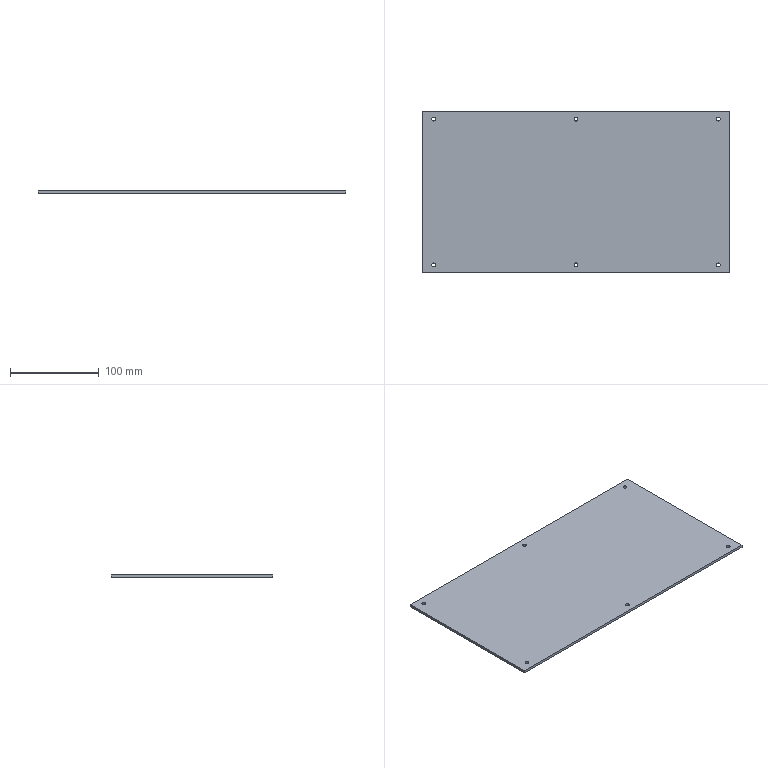Part | SolidWorks | features Cut 1, Extrusion 1 | 1 solid | 18 faces | box 346 x 182 x 3 mm | volume 188642 mm3 | cylinder 12 | plane 6 | commonest cylinder face diameters 4.4 x12
STEP:
#1=CARTESIAN_POINT('',(157.8,-82.,3.));
#2=VERTEX_POINT('',#1);
#3=CARTESIAN_POINT('',(162.2,-82.,3.));
#4=VERTEX_POINT('',#3);
#5=CARTESIAN_POINT('',(160.,-82.,3.));
#6=DIRECTION('',(0.,0.,1.));
#7=DIRECTION('',(1.,0.,0.));
#8=AXIS2_PLACEMENT_3D('',#5,#6,#7);
#9=CIRCLE('',#8,2.2);
#10=EDGE_CURVE('',#2,#4,#9,.T.);
#11=ORIENTED_EDGE('',*,*,#10,.T.);
#12=CARTESIAN_POINT('',(162.2,-82.,0.));
#13=VERTEX_POINT('',#12);
#14=CARTESIAN_POINT('',(162.2,-82.,10.));
#15=DIRECTION('',(0.,0.,-1.));
#16=VECTOR('',#15,1000.);
#17=LINE('',#14,#16);
#18=EDGE_CURVE('',#4,#13,#17,.T.);
#19=ORIENTED_EDGE('',*,*,#18,.T.);
#20=CARTESIAN_POINT('',(157.8,-82.,0.));
#21=VERTEX_POINT('',#20);
#22=CARTESIAN_POINT('',(160.,-82.,0.));
#23=DIRECTION('',(0.,0.,-1.));
#24=DIRECTION('',(-1.,0.,0.));
#25=AXIS2_PLACEMENT_3D('',#22,#23,#24);
#26=CIRCLE('',#25,2.2);
#27=EDGE_CURVE('',#13,#21,#26,.T.);
#28=ORIENTED_EDGE('',*,*,#27,.T.);
#29=CARTESIAN_POINT('',(157.8,-82.,10.));
#30=DIRECTION('',(0.,0.,-1.));
#31=VECTOR('',#30,1000.);
#32=LINE('',#29,#31);
#33=EDGE_CURVE('',#2,#21,#32,.T.);
#34=ORIENTED_EDGE('',*,*,#33,.F.);
#35=EDGE_LOOP('',(#11,#19,#28,#34));
#36=FACE_OUTER_BOUND('',#35,.T.);
#37=CARTESIAN_POINT('',(160.,-82.,10.));
#38=DIRECTION('',(0.,0.,-1.));
#39=DIRECTION('',(-1.,0.,0.));
#40=AXIS2_PLACEMENT_3D('',#37,#38,#39);
#41=CYLINDRICAL_SURFACE('',#40,2.2);
#42=ADVANCED_FACE('',(#36),#41,.F.);
#43=CARTESIAN_POINT('',(-162.2,-82.,3.));
#44=VERTEX_POINT('',#43);
#45=CARTESIAN_POINT('',(-157.8,-82.,3.));
#46=VERTEX_POINT('',#45);
#47=CARTESIAN_POINT('',(-160.,-82.,3.));
#48=DIRECTION('',(0.,0.,1.));
#49=DIRECTION('',(1.,0.,0.));
#50=AXIS2_PLACEMENT_3D('',#47,#48,#49);
#51=CIRCLE('',#50,2.2);
#52=EDGE_CURVE('',#44,#46,#51,.T.);
#53=ORIENTED_EDGE('',*,*,#52,.T.);
#54=CARTESIAN_POINT('',(-157.8,-82.,0.));
#55=VERTEX_POINT('',#54);
#56=CARTESIAN_POINT('',(-157.8,-82.,10.));
#57=DIRECTION('',(0.,0.,-1.));
#58=VECTOR('',#57,1000.);
#59=LINE('',#56,#58);
#60=EDGE_CURVE('',#46,#55,#59,.T.);
#61=ORIENTED_EDGE('',*,*,#60,.T.);
#62=CARTESIAN_POINT('',(-162.2,-82.,0.));
#63=VERTEX_POINT('',#62);
#64=CARTESIAN_POINT('',(-160.,-82.,0.));
#65=DIRECTION('',(0.,0.,-1.));
#66=DIRECTION('',(-1.,0.,0.));
#67=AXIS2_PLACEMENT_3D('',#64,#65,#66);
#68=CIRCLE('',#67,2.2);
#69=EDGE_CURVE('',#55,#63,#68,.T.);
#70=ORIENTED_EDGE('',*,*,#69,.T.);
#71=CARTESIAN_POINT('',(-162.2,-82.,10.));
#72=DIRECTION('',(0.,0.,-1.));
#73=VECTOR('',#72,1000.);
#74=LINE('',#71,#73);
#75=EDGE_CURVE('',#44,#63,#74,.T.);
#76=ORIENTED_EDGE('',*,*,#75,.F.);
#77=EDGE_LOOP('',(#53,#61,#70,#76));
#78=FACE_OUTER_BOUND('',#77,.T.);
#79=CARTESIAN_POINT('',(-160.,-82.,10.));
#80=DIRECTION('',(0.,0.,-1.));
#81=DIRECTION('',(-1.,0.,0.));
#82=AXIS2_PLACEMENT_3D('',#79,#80,#81);
#83=CYLINDRICAL_SURFACE('',#82,2.2);
#84=ADVANCED_FACE('',(#78),#83,.F.);
#85=CARTESIAN_POINT('',(-2.2,-82.,3.));
#86=VERTEX_POINT('',#85);
#87=CARTESIAN_POINT('',(2.2,-82.,3.));
#88=VERTEX_POINT('',#87);
#89=CARTESIAN_POINT('',(0.,-82.,3.));
#90=DIRECTION('',(0.,0.,1.));
#91=DIRECTION('',(1.,0.,0.));
#92=AXIS2_PLACEMENT_3D('',#89,#90,#91);
#93=CIRCLE('',#92,2.2);
#94=EDGE_CURVE('',#86,#88,#93,.T.);
#95=ORIENTED_EDGE('',*,*,#94,.T.);
#96=CARTESIAN_POINT('',(2.2,-82.,0.));
#97=VERTEX_POINT('',#96);
#98=CARTESIAN_POINT('',(2.2,-82.,10.));
#99=DIRECTION('',(0.,0.,-1.));
#100=VECTOR('',#99,1000.);
#101=LINE('',#98,#100);
#102=EDGE_CURVE('',#88,#97,#101,.T.);
#103=ORIENTED_EDGE('',*,*,#102,.T.);
#104=CARTESIAN_POINT('',(-2.2,-82.,0.));
#105=VERTEX_POINT('',#104);
#106=CARTESIAN_POINT('',(0.,-82.,0.));
#107=DIRECTION('',(0.,0.,-1.));
#108=DIRECTION('',(-1.,0.,0.));
#109=AXIS2_PLACEMENT_3D('',#106,#107,#108);
#110=CIRCLE('',#109,2.2);
#111=EDGE_CURVE('',#97,#105,#110,.T.);
#112=ORIENTED_EDGE('',*,*,#111,.T.);
#113=CARTESIAN_POINT('',(-2.2,-82.,10.));
#114=DIRECTION('',(0.,0.,-1.));
#115=VECTOR('',#114,1000.);
#116=LINE('',#113,#115);
#117=EDGE_CURVE('',#86,#105,#116,.T.);
#118=ORIENTED_EDGE('',*,*,#117,.F.);
#119=EDGE_LOOP('',(#95,#103,#112,#118));
#120=FACE_OUTER_BOUND('',#119,.T.);
#121=CARTESIAN_POINT('',(0.,-82.,10.));
#122=DIRECTION('',(0.,0.,-1.));
#123=DIRECTION('',(-1.,0.,0.));
#124=AXIS2_PLACEMENT_3D('',#121,#122,#123);
#125=CYLINDRICAL_SURFACE('',#124,2.2);
#126=ADVANCED_FACE('',(#120),#125,.F.);
#127=CARTESIAN_POINT('',(-162.2,82.,3.));
#128=VERTEX_POINT('',#127);
#129=CARTESIAN_POINT('',(-157.8,82.,3.));
#130=VERTEX_POINT('',#129);
#131=CARTESIAN_POINT('',(-160.,82.,3.));
#132=DIRECTION('',(0.,0.,1.));
#133=DIRECTION('',(1.,0.,0.));
#134=AXIS2_PLACEMENT_3D('',#131,#132,#133);
#135=CIRCLE('',#134,2.2);
#136=EDGE_CURVE('',#128,#130,#135,.T.);
#137=ORIENTED_EDGE('',*,*,#136,.T.);
#138=CARTESIAN_POINT('',(-157.8,82.,0.));
#139=VERTEX_POINT('',#138);
#140=CARTESIAN_POINT('',(-157.8,82.,10.));
#141=DIRECTION('',(0.,0.,-1.));
#142=VECTOR('',#141,1000.);
#143=LINE('',#140,#142);
#144=EDGE_CURVE('',#130,#139,#143,.T.);
#145=ORIENTED_EDGE('',*,*,#144,.T.);
#146=CARTESIAN_POINT('',(-162.2,82.,0.));
#147=VERTEX_POINT('',#146);
#148=CARTESIAN_POINT('',(-160.,82.,0.));
#149=DIRECTION('',(0.,0.,-1.));
#150=DIRECTION('',(-1.,0.,0.));
#151=AXIS2_PLACEMENT_3D('',#148,#149,#150);
#152=CIRCLE('',#151,2.2);
#153=EDGE_CURVE('',#139,#147,#152,.T.);
#154=ORIENTED_EDGE('',*,*,#153,.T.);
#155=CARTESIAN_POINT('',(-162.2,82.,10.));
#156=DIRECTION('',(0.,0.,-1.));
#157=VECTOR('',#156,1000.);
#158=LINE('',#155,#157);
#159=EDGE_CURVE('',#128,#147,#158,.T.);
#160=ORIENTED_EDGE('',*,*,#159,.F.);
#161=EDGE_LOOP('',(#137,#145,#154,#160));
#162=FACE_OUTER_BOUND('',#161,.T.);
#163=CARTESIAN_POINT('',(-160.,82.,10.));
#164=DIRECTION('',(0.,0.,-1.));
#165=DIRECTION('',(-1.,0.,0.));
#166=AXIS2_PLACEMENT_3D('',#163,#164,#165);
#167=CYLINDRICAL_SURFACE('',#166,2.2);
#168=ADVANCED_FACE('',(#162),#167,.F.);
#169=CARTESIAN_POINT('',(-2.2,82.,3.));
#170=VERTEX_POINT('',#169);
#171=CARTESIAN_POINT('',(2.2,82.,3.));
#172=VERTEX_POINT('',#171);
#173=CARTESIAN_POINT('',(0.,82.,3.));
#174=DIRECTION('',(0.,0.,1.));
#175=DIRECTION('',(1.,0.,0.));
#176=AXIS2_PLACEMENT_3D('',#173,#174,#175);
#177=CIRCLE('',#176,2.2);
#178=EDGE_CURVE('',#170,#172,#177,.T.);
#179=ORIENTED_EDGE('',*,*,#178,.T.);
#180=CARTESIAN_POINT('',(2.2,82.,0.));
#181=VERTEX_POINT('',#180);
#182=CARTESIAN_POINT('',(2.2,82.,10.));
#183=DIRECTION('',(0.,0.,-1.));
#184=VECTOR('',#183,1000.);
#185=LINE('',#182,#184);
#186=EDGE_CURVE('',#172,#181,#185,.T.);
#187=ORIENTED_EDGE('',*,*,#186,.T.);
#188=CARTESIAN_POINT('',(-2.2,82.,0.));
#189=VERTEX_POINT('',#188);
#190=CARTESIAN_POINT('',(0.,82.,0.));
#191=DIRECTION('',(0.,0.,-1.));
#192=DIRECTION('',(-1.,0.,0.));
#193=AXIS2_PLACEMENT_3D('',#190,#191,#192);
#194=CIRCLE('',#193,2.2);
#195=EDGE_CURVE('',#181,#189,#194,.T.);
#196=ORIENTED_EDGE('',*,*,#195,.T.);
#197=CARTESIAN_POINT('',(-2.2,82.,10.));
#198=DIRECTION('',(0.,0.,-1.));
#199=VECTOR('',#198,1000.);
#200=LINE('',#197,#199);
#201=EDGE_CURVE('',#170,#189,#200,.T.);
#202=ORIENTED_EDGE('',*,*,#201,.F.);
#203=EDGE_LOOP('',(#179,#187,#196,#202));
#204=FACE_OUTER_BOUND('',#203,.T.);
#205=CARTESIAN_POINT('',(0.,82.,10.));
#206=DIRECTION('',(0.,0.,-1.));
#207=DIRECTION('',(-1.,0.,0.));
#208=AXIS2_PLACEMENT_3D('',#205,#206,#207);
#209=CYLINDRICAL_SURFACE('',#208,2.2);
#210=ADVANCED_FACE('',(#204),#209,.F.);
#211=CARTESIAN_POINT('',(157.8,82.,3.));
#212=VERTEX_POINT('',#211);
#213=CARTESIAN_POINT('',(162.2,82.,3.));
#214=VERTEX_POINT('',#213);
#215=CARTESIAN_POINT('',(160.,82.,3.));
#216=DIRECTION('',(0.,0.,1.));
#217=DIRECTION('',(1.,0.,0.));
#218=AXIS2_PLACEMENT_3D('',#215,#216,#217);
#219=CIRCLE('',#218,2.2);
#220=EDGE_CURVE('',#212,#214,#219,.T.);
#221=ORIENTED_EDGE('',*,*,#220,.T.);
#222=CARTESIAN_POINT('',(162.2,82.,0.));
#223=VERTEX_POINT('',#222);
#224=CARTESIAN_POINT('',(162.2,82.,10.));
#225=DIRECTION('',(0.,0.,-1.));
#226=VECTOR('',#225,1000.);
#227=LINE('',#224,#226);
#228=EDGE_CURVE('',#214,#223,#227,.T.);
#229=ORIENTED_EDGE('',*,*,#228,.T.);
#230=CARTESIAN_POINT('',(157.8,82.,0.));
#231=VERTEX_POINT('',#230);
#232=CARTESIAN_POINT('',(160.,82.,0.));
#233=DIRECTION('',(0.,0.,-1.));
#234=DIRECTION('',(-1.,0.,0.));
#235=AXIS2_PLACEMENT_3D('',#232,#233,#234);
#236=CIRCLE('',#235,2.2);
#237=EDGE_CURVE('',#223,#231,#236,.T.);
#238=ORIENTED_EDGE('',*,*,#237,.T.);
#239=CARTESIAN_POINT('',(157.8,82.,10.));
#240=DIRECTION('',(0.,0.,-1.));
#241=VECTOR('',#240,1000.);
#242=LINE('',#239,#241);
#243=EDGE_CURVE('',#212,#231,#242,.T.);
#244=ORIENTED_EDGE('',*,*,#243,.F.);
#245=EDGE_LOOP('',(#221,#229,#238,#244));
#246=FACE_OUTER_BOUND('',#245,.T.);
#247=CARTESIAN_POINT('',(160.,82.,10.));
#248=DIRECTION('',(0.,0.,-1.));
#249=DIRECTION('',(-1.,0.,0.));
#250=AXIS2_PLACEMENT_3D('',#247,#248,#249);
#251=CYLINDRICAL_SURFACE('',#250,2.2);
#252=ADVANCED_FACE('',(#246),#251,.F.);
#253=CARTESIAN_POINT('',(-173.,91.,0.));
#254=VERTEX_POINT('',#253);
#255=CARTESIAN_POINT('',(-173.,-91.,0.));
#256=VERTEX_POINT('',#255);
#257=CARTESIAN_POINT('',(-173.,-91.,0.));
#258=DIRECTION('',(0.,-1.,0.));
#259=VECTOR('',#258,1000.);
#260=LINE('',#257,#259);
#261=EDGE_CURVE('',#254,#256,#260,.T.);
#262=ORIENTED_EDGE('',*,*,#261,.T.);
#263=CARTESIAN_POINT('',(-173.,-91.,3.));
#264=VERTEX_POINT('',#263);
#265=CARTESIAN_POINT('',(-173.,-91.,3.));
#266=DIRECTION('',(0.,0.,-1.));
#267=VECTOR('',#266,1000.);
#268=LINE('',#265,#267);
#269=EDGE_CURVE('',#264,#256,#268,.T.);
#270=ORIENTED_EDGE('',*,*,#269,.F.);
#271=CARTESIAN_POINT('',(-173.,91.,3.));
#272=VERTEX_POINT('',#271);
#273=CARTESIAN_POINT('',(-173.,-91.,3.));
#274=DIRECTION('',(0.,-1.,0.));
#275=VECTOR('',#274,1000.);
#276=LINE('',#273,#275);
#277=EDGE_CURVE('',#272,#264,#276,.T.);
#278=ORIENTED_EDGE('',*,*,#277,.F.);
#279=CARTESIAN_POINT('',(-173.,91.,3.));
#280=DIRECTION('',(0.,0.,-1.));
#281=VECTOR('',#280,1000.);
#282=LINE('',#279,#281);
#283=EDGE_CURVE('',#272,#254,#282,.T.);
#284=ORIENTED_EDGE('',*,*,#283,.T.);
#285=EDGE_LOOP('',(#262,#270,#278,#284));
#286=FACE_OUTER_BOUND('',#285,.T.);
#287=CARTESIAN_POINT('',(-173.,-91.,3.));
#288=DIRECTION('',(1.,0.,0.));
#289=DIRECTION('',(0.,0.,-1.));
#290=AXIS2_PLACEMENT_3D('',#287,#288,#289);
#291=PLANE('',#290);
#292=ADVANCED_FACE('',(#286),#291,.F.);
#293=CARTESIAN_POINT('',(173.,-91.,0.));
#294=VERTEX_POINT('',#293);
#295=CARTESIAN_POINT('',(173.,-91.,0.));
#296=DIRECTION('',(1.,0.,0.));
#297=VECTOR('',#296,1000.);
#298=LINE('',#295,#297);
#299=EDGE_CURVE('',#256,#294,#298,.T.);
#300=ORIENTED_EDGE('',*,*,#299,.T.);
#301=CARTESIAN_POINT('',(173.,-91.,3.));
#302=VERTEX_POINT('',#301);
#303=CARTESIAN_POINT('',(173.,-91.,3.));
#304=DIRECTION('',(0.,0.,-1.));
#305=VECTOR('',#304,1000.);
#306=LINE('',#303,#305);
#307=EDGE_CURVE('',#302,#294,#306,.T.);
#308=ORIENTED_EDGE('',*,*,#307,.F.);
#309=CARTESIAN_POINT('',(173.,-91.,3.));
#310=DIRECTION('',(1.,0.,0.));
#311=VECTOR('',#310,1000.);
#312=LINE('',#309,#311);
#313=EDGE_CURVE('',#264,#302,#312,.T.);
#314=ORIENTED_EDGE('',*,*,#313,.F.);
#315=ORIENTED_EDGE('',*,*,#269,.T.);
#316=EDGE_LOOP('',(#300,#308,#314,#315));
#317=FACE_OUTER_BOUND('',#316,.T.);
#318=CARTESIAN_POINT('',(173.,-91.,3.));
#319=DIRECTION('',(0.,1.,0.));
#320=DIRECTION('',(-1.,0.,0.));
#321=AXIS2_PLACEMENT_3D('',#318,#319,#320);
#322=PLANE('',#321);
#323=ADVANCED_FACE('',(#317),#322,.F.);
#324=CARTESIAN_POINT('',(173.,91.,0.));
#325=VERTEX_POINT('',#324);
#326=CARTESIAN_POINT('',(173.,-91.,0.));
#327=DIRECTION('',(0.,1.,0.));
#328=VECTOR('',#327,1000.);
#329=LINE('',#326,#328);
#330=EDGE_CURVE('',#294,#325,#329,.T.);
#331=ORIENTED_EDGE('',*,*,#330,.T.);
#332=CARTESIAN_POINT('',(173.,91.,3.));
#333=VERTEX_POINT('',#332);
#334=CARTESIAN_POINT('',(173.,91.,3.));
#335=DIRECTION('',(0.,0.,-1.));
#336=VECTOR('',#335,1000.);
#337=LINE('',#334,#336);
#338=EDGE_CURVE('',#333,#325,#337,.T.);
#339=ORIENTED_EDGE('',*,*,#338,.F.);
#340=CARTESIAN_POINT('',(173.,-91.,3.));
#341=DIRECTION('',(0.,1.,0.));
#342=VECTOR('',#341,1000.);
#343=LINE('',#340,#342);
#344=EDGE_CURVE('',#302,#333,#343,.T.);
#345=ORIENTED_EDGE('',*,*,#344,.F.);
#346=ORIENTED_EDGE('',*,*,#307,.T.);
#347=EDGE_LOOP('',(#331,#339,#345,#346));
#348=FACE_OUTER_BOUND('',#347,.T.);
#349=CARTESIAN_POINT('',(173.,-91.,3.));
#350=DIRECTION('',(-1.,0.,0.));
#351=DIRECTION('',(0.,0.,1.));
#352=AXIS2_PLACEMENT_3D('',#349,#350,#351);
#353=PLANE('',#352);
#354=ADVANCED_FACE('',(#348),#353,.F.);
#355=CARTESIAN_POINT('',(173.,91.,0.));
#356=DIRECTION('',(-1.,0.,0.));
#357=VECTOR('',#356,1000.);
#358=LINE('',#355,#357);
#359=EDGE_CURVE('',#325,#254,#358,.T.);
#360=ORIENTED_EDGE('',*,*,#359,.T.);
#361=ORIENTED_EDGE('',*,*,#283,.F.);
#362=CARTESIAN_POINT('',(173.,91.,3.));
#363=DIRECTION('',(-1.,0.,0.));
#364=VECTOR('',#363,1000.);
#365=LINE('',#362,#364);
#366=EDGE_CURVE('',#333,#272,#365,.T.);
#367=ORIENTED_EDGE('',*,*,#366,.F.);
#368=ORIENTED_EDGE('',*,*,#338,.T.);
#369=EDGE_LOOP('',(#360,#361,#367,#368));
#370=FACE_OUTER_BOUND('',#369,.T.);
#371=CARTESIAN_POINT('',(173.,91.,3.));
#372=DIRECTION('',(0.,-1.,0.));
#373=DIRECTION('',(1.,0.,0.));
#374=AXIS2_PLACEMENT_3D('',#371,#372,#373);
#375=PLANE('',#374);
#376=ADVANCED_FACE('',(#370),#375,.F.);
#377=ORIENTED_EDGE('',*,*,#10,.F.);
#378=CARTESIAN_POINT('',(160.,-82.,3.));
#379=DIRECTION('',(0.,0.,1.));
#380=DIRECTION('',(1.,0.,0.));
#381=AXIS2_PLACEMENT_3D('',#378,#379,#380);
#382=CIRCLE('',#381,2.2);
#383=EDGE_CURVE('',#4,#2,#382,.T.);
#384=ORIENTED_EDGE('',*,*,#383,.F.);
#385=EDGE_LOOP('',(#377,#384));
#386=FACE_BOUND('',#385,.T.);
#387=ORIENTED_EDGE('',*,*,#52,.F.);
#388=CARTESIAN_POINT('',(-160.,-82.,3.));
#389=DIRECTION('',(0.,0.,1.));
#390=DIRECTION('',(1.,0.,0.));
#391=AXIS2_PLACEMENT_3D('',#388,#389,#390);
#392=CIRCLE('',#391,2.2);
#393=EDGE_CURVE('',#46,#44,#392,.T.);
#394=ORIENTED_EDGE('',*,*,#393,.F.);
#395=EDGE_LOOP('',(#387,#394));
#396=FACE_BOUND('',#395,.T.);
#397=ORIENTED_EDGE('',*,*,#94,.F.);
#398=CARTESIAN_POINT('',(0.,-82.,3.));
#399=DIRECTION('',(0.,0.,1.));
#400=DIRECTION('',(1.,0.,0.));
#401=AXIS2_PLACEMENT_3D('',#398,#399,#400);
#402=CIRCLE('',#401,2.2);
#403=EDGE_CURVE('',#88,#86,#402,.T.);
#404=ORIENTED_EDGE('',*,*,#403,.F.);
#405=EDGE_LOOP('',(#397,#404));
#406=FACE_BOUND('',#405,.T.);
#407=ORIENTED_EDGE('',*,*,#136,.F.);
#408=CARTESIAN_POINT('',(-160.,82.,3.));
#409=DIRECTION('',(0.,0.,1.));
#410=DIRECTION('',(1.,0.,0.));
#411=AXIS2_PLACEMENT_3D('',#408,#409,#410);
#412=CIRCLE('',#411,2.2);
#413=EDGE_CURVE('',#130,#128,#412,.T.);
#414=ORIENTED_EDGE('',*,*,#413,.F.);
#415=EDGE_LOOP('',(#407,#414));
#416=FACE_BOUND('',#415,.T.);
#417=ORIENTED_EDGE('',*,*,#178,.F.);
#418=CARTESIAN_POINT('',(0.,82.,3.));
#419=DIRECTION('',(0.,0.,1.));
#420=DIRECTION('',(1.,0.,0.));
#421=AXIS2_PLACEMENT_3D('',#418,#419,#420);
#422=CIRCLE('',#421,2.2);
#423=EDGE_CURVE('',#172,#170,#422,.T.);
#424=ORIENTED_EDGE('',*,*,#423,.F.);
#425=EDGE_LOOP('',(#417,#424));
#426=FACE_BOUND('',#425,.T.);
#427=ORIENTED_EDGE('',*,*,#220,.F.);
#428=CARTESIAN_POINT('',(160.,82.,3.));
#429=DIRECTION('',(0.,0.,1.));
#430=DIRECTION('',(1.,0.,0.));
#431=AXIS2_PLACEMENT_3D('',#428,#429,#430);
#432=CIRCLE('',#431,2.2);
#433=EDGE_CURVE('',#214,#212,#432,.T.);
#434=ORIENTED_EDGE('',*,*,#433,.F.);
#435=EDGE_LOOP('',(#427,#434));
#436=FACE_BOUND('',#435,.T.);
#437=ORIENTED_EDGE('',*,*,#277,.T.);
#438=ORIENTED_EDGE('',*,*,#313,.T.);
#439=ORIENTED_EDGE('',*,*,#344,.T.);
#440=ORIENTED_EDGE('',*,*,#366,.T.);
#441=EDGE_LOOP('',(#437,#438,#439,#440));
#442=FACE_OUTER_BOUND('',#441,.T.);
#443=CARTESIAN_POINT('',(0.,0.,3.));
#444=DIRECTION('',(0.,0.,1.));
#445=DIRECTION('',(1.,0.,0.));
#446=AXIS2_PLACEMENT_3D('',#443,#444,#445);
#447=PLANE('',#446);
#448=ADVANCED_FACE('',(#386,#396,#406,#416,#426,#436,#442),#447,.T.);
#449=CARTESIAN_POINT('',(160.,-82.,0.));
#450=DIRECTION('',(0.,0.,-1.));
#451=DIRECTION('',(-1.,0.,0.));
#452=AXIS2_PLACEMENT_3D('',#449,#450,#451);
#453=CIRCLE('',#452,2.2);
#454=EDGE_CURVE('',#21,#13,#453,.T.);
#455=ORIENTED_EDGE('',*,*,#454,.F.);
#456=ORIENTED_EDGE('',*,*,#27,.F.);
#457=EDGE_LOOP('',(#455,#456));
#458=FACE_BOUND('',#457,.T.);
#459=CARTESIAN_POINT('',(-160.,-82.,0.));
#460=DIRECTION('',(0.,0.,-1.));
#461=DIRECTION('',(-1.,0.,0.));
#462=AXIS2_PLACEMENT_3D('',#459,#460,#461);
#463=CIRCLE('',#462,2.2);
#464=EDGE_CURVE('',#63,#55,#463,.T.);
#465=ORIENTED_EDGE('',*,*,#464,.F.);
#466=ORIENTED_EDGE('',*,*,#69,.F.);
#467=EDGE_LOOP('',(#465,#466));
#468=FACE_BOUND('',#467,.T.);
#469=CARTESIAN_POINT('',(0.,-82.,0.));
#470=DIRECTION('',(0.,0.,-1.));
#471=DIRECTION('',(-1.,0.,0.));
#472=AXIS2_PLACEMENT_3D('',#469,#470,#471);
#473=CIRCLE('',#472,2.2);
#474=EDGE_CURVE('',#105,#97,#473,.T.);
#475=ORIENTED_EDGE('',*,*,#474,.F.);
#476=ORIENTED_EDGE('',*,*,#111,.F.);
#477=EDGE_LOOP('',(#475,#476));
#478=FACE_BOUND('',#477,.T.);
#479=CARTESIAN_POINT('',(-160.,82.,0.));
#480=DIRECTION('',(0.,0.,-1.));
#481=DIRECTION('',(-1.,0.,0.));
#482=AXIS2_PLACEMENT_3D('',#479,#480,#481);
#483=CIRCLE('',#482,2.2);
#484=EDGE_CURVE('',#147,#139,#483,.T.);
#485=ORIENTED_EDGE('',*,*,#484,.F.);
#486=ORIENTED_EDGE('',*,*,#153,.F.);
#487=EDGE_LOOP('',(#485,#486));
#488=FACE_BOUND('',#487,.T.);
#489=CARTESIAN_POINT('',(0.,82.,0.));
#490=DIRECTION('',(0.,0.,-1.));
#491=DIRECTION('',(-1.,0.,0.));
#492=AXIS2_PLACEMENT_3D('',#489,#490,#491);
#493=CIRCLE('',#492,2.2);
#494=EDGE_CURVE('',#189,#181,#493,.T.);
#495=ORIENTED_EDGE('',*,*,#494,.F.);
#496=ORIENTED_EDGE('',*,*,#195,.F.);
#497=EDGE_LOOP('',(#495,#496));
#498=FACE_BOUND('',#497,.T.);
#499=CARTESIAN_POINT('',(160.,82.,0.));
#500=DIRECTION('',(0.,0.,-1.));
#501=DIRECTION('',(-1.,0.,0.));
#502=AXIS2_PLACEMENT_3D('',#499,#500,#501);
#503=CIRCLE('',#502,2.2);
#504=EDGE_CURVE('',#231,#223,#503,.T.);
#505=ORIENTED_EDGE('',*,*,#504,.F.);
#506=ORIENTED_EDGE('',*,*,#237,.F.);
#507=EDGE_LOOP('',(#505,#506));
#508=FACE_BOUND('',#507,.T.);
#509=ORIENTED_EDGE('',*,*,#261,.F.);
#510=ORIENTED_EDGE('',*,*,#359,.F.);
#511=ORIENTED_EDGE('',*,*,#330,.F.);
#512=ORIENTED_EDGE('',*,*,#299,.F.);
#513=EDGE_LOOP('',(#509,#510,#511,#512));
#514=FACE_OUTER_BOUND('',#513,.T.);
#515=CARTESIAN_POINT('',(0.,0.,0.));
#516=DIRECTION('',(0.,0.,1.));
#517=DIRECTION('',(1.,0.,0.));
#518=AXIS2_PLACEMENT_3D('',#515,#516,#517);
#519=PLANE('',#518);
#520=ADVANCED_FACE('',(#458,#468,#478,#488,#498,#508,#514),#519,.F.);
#521=ORIENTED_EDGE('',*,*,#228,.F.);
#522=ORIENTED_EDGE('',*,*,#433,.T.);
#523=ORIENTED_EDGE('',*,*,#243,.T.);
#524=ORIENTED_EDGE('',*,*,#504,.T.);
#525=EDGE_LOOP('',(#521,#522,#523,#524));
#526=FACE_OUTER_BOUND('',#525,.T.);
#527=CARTESIAN_POINT('',(160.,82.,10.));
#528=DIRECTION('',(0.,0.,-1.));
#529=DIRECTION('',(-1.,0.,0.));
#530=AXIS2_PLACEMENT_3D('',#527,#528,#529);
#531=CYLINDRICAL_SURFACE('',#530,2.2);
#532=ADVANCED_FACE('',(#526),#531,.F.);
#533=ORIENTED_EDGE('',*,*,#186,.F.);
#534=ORIENTED_EDGE('',*,*,#423,.T.);
#535=ORIENTED_EDGE('',*,*,#201,.T.);
#536=ORIENTED_EDGE('',*,*,#494,.T.);
#537=EDGE_LOOP('',(#533,#534,#535,#536));
#538=FACE_OUTER_BOUND('',#537,.T.);
#539=CARTESIAN_POINT('',(0.,82.,10.));
#540=DIRECTION('',(0.,0.,-1.));
#541=DIRECTION('',(-1.,0.,0.));
#542=AXIS2_PLACEMENT_3D('',#539,#540,#541);
#543=CYLINDRICAL_SURFACE('',#542,2.2);
#544=ADVANCED_FACE('',(#538),#543,.F.);
#545=ORIENTED_EDGE('',*,*,#144,.F.);
#546=ORIENTED_EDGE('',*,*,#413,.T.);
#547=ORIENTED_EDGE('',*,*,#159,.T.);
#548=ORIENTED_EDGE('',*,*,#484,.T.);
#549=EDGE_LOOP('',(#545,#546,#547,#548));
#550=FACE_OUTER_BOUND('',#549,.T.);
#551=CARTESIAN_POINT('',(-160.,82.,10.));
#552=DIRECTION('',(0.,0.,-1.));
#553=DIRECTION('',(-1.,0.,0.));
#554=AXIS2_PLACEMENT_3D('',#551,#552,#553);
#555=CYLINDRICAL_SURFACE('',#554,2.2);
#556=ADVANCED_FACE('',(#550),#555,.F.);
#557=ORIENTED_EDGE('',*,*,#102,.F.);
#558=ORIENTED_EDGE('',*,*,#403,.T.);
#559=ORIENTED_EDGE('',*,*,#117,.T.);
#560=ORIENTED_EDGE('',*,*,#474,.T.);
#561=EDGE_LOOP('',(#557,#558,#559,#560));
#562=FACE_OUTER_BOUND('',#561,.T.);
#563=CARTESIAN_POINT('',(0.,-82.,10.));
#564=DIRECTION('',(0.,0.,-1.));
#565=DIRECTION('',(-1.,0.,0.));
#566=AXIS2_PLACEMENT_3D('',#563,#564,#565);
#567=CYLINDRICAL_SURFACE('',#566,2.2);
#568=ADVANCED_FACE('',(#562),#567,.F.);
#569=ORIENTED_EDGE('',*,*,#60,.F.);
#570=ORIENTED_EDGE('',*,*,#393,.T.);
#571=ORIENTED_EDGE('',*,*,#75,.T.);
#572=ORIENTED_EDGE('',*,*,#464,.T.);
#573=EDGE_LOOP('',(#569,#570,#571,#572));
#574=FACE_OUTER_BOUND('',#573,.T.);
#575=CARTESIAN_POINT('',(-160.,-82.,10.));
#576=DIRECTION('',(0.,0.,-1.));
#577=DIRECTION('',(-1.,0.,0.));
#578=AXIS2_PLACEMENT_3D('',#575,#576,#577);
#579=CYLINDRICAL_SURFACE('',#578,2.2);
#580=ADVANCED_FACE('',(#574),#579,.F.);
#581=ORIENTED_EDGE('',*,*,#18,.F.);
#582=ORIENTED_EDGE('',*,*,#383,.T.);
#583=ORIENTED_EDGE('',*,*,#33,.T.);
#584=ORIENTED_EDGE('',*,*,#454,.T.);
#585=EDGE_LOOP('',(#581,#582,#583,#584));
#586=FACE_OUTER_BOUND('',#585,.T.);
#587=CARTESIAN_POINT('',(160.,-82.,10.));
#588=DIRECTION('',(0.,0.,-1.));
#589=DIRECTION('',(-1.,0.,0.));
#590=AXIS2_PLACEMENT_3D('',#587,#588,#589);
#591=CYLINDRICAL_SURFACE('',#590,2.2);
#592=ADVANCED_FACE('',(#586),#591,.F.);
#593=CLOSED_SHELL('',(#42,#84,#126,#168,#210,#252,#292,#323,#354,#376,#448,#520,#532,#544,#556,#568,#580,#592));
#594=MANIFOLD_SOLID_BREP('',#593);
#595=CARTESIAN_POINT('',(0.,0.,0.));
#596=DIRECTION('',(0.,0.,1.));
#597=DIRECTION('',(1.,0.,0.));
#598=AXIS2_PLACEMENT_3D('',#595,#596,#597);
#599=(LENGTH_UNIT()NAMED_UNIT(*)SI_UNIT(.MILLI.,.METRE.));
#600=UNCERTAINTY_MEASURE_WITH_UNIT(LENGTH_MEASURE(0.00001),#599,'','');
#601=(NAMED_UNIT(*)PLANE_ANGLE_UNIT()SI_UNIT($,.RADIAN.));
#602=(NAMED_UNIT(*)SI_UNIT($,.STERADIAN.)SOLID_ANGLE_UNIT());
#603=(GEOMETRIC_REPRESENTATION_CONTEXT(3)GLOBAL_UNCERTAINTY_ASSIGNED_CONTEXT((#600))GLOBAL_UNIT_ASSIGNED_CONTEXT((#599,#601,#602))REPRESENTATION_CONTEXT('',''));
#604=ADVANCED_BREP_SHAPE_REPRESENTATION('',(#594,#598),#603);